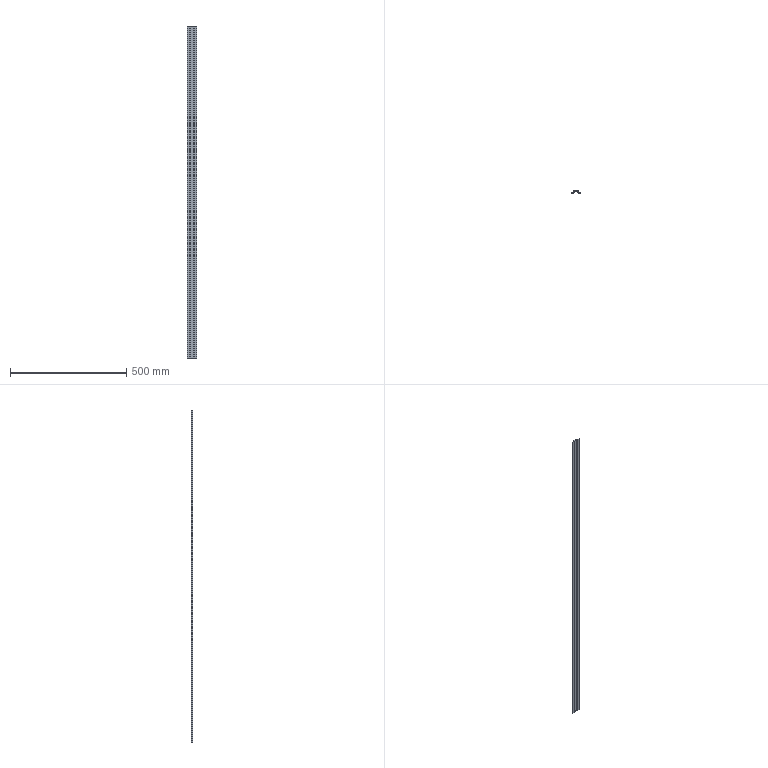Part | SolidWorks | features FlatPattern 1, SMBaseFlange 1, SheetMetal 1 | 1 solid | 38 faces | box 40 x 6.5 x 1430 mm | volume 103752 mm3 | plane 30 | cylinder 8 | commonest cylinder face diameters 0.4 x4 3.4 x4
STEP:
#1=CARTESIAN_POINT('',(10.,0.2,715.));
#2=VERTEX_POINT('',#1);
#3=CARTESIAN_POINT('',(11.5,0.2,715.));
#4=VERTEX_POINT('',#3);
#5=CARTESIAN_POINT('',(10.,0.2,715.));
#6=DIRECTION('',(1.,0.,0.));
#7=VECTOR('',#6,1000.);
#8=LINE('',#5,#7);
#9=EDGE_CURVE('',#2,#4,#8,.T.);
#10=ORIENTED_EDGE('',*,*,#9,.F.);
#11=CARTESIAN_POINT('',(9.8,0.,715.));
#12=VERTEX_POINT('',#11);
#13=CARTESIAN_POINT('',(9.8,0.2,715.));
#14=DIRECTION('',(0.,0.,1.));
#15=DIRECTION('',(-1.,0.,0.));
#16=AXIS2_PLACEMENT_3D('',#13,#14,#15);
#17=CIRCLE('',#16,0.2);
#18=EDGE_CURVE('',#12,#2,#17,.T.);
#19=ORIENTED_EDGE('',*,*,#18,.F.);
#20=CARTESIAN_POINT('',(9.8,-1.5,715.));
#21=VERTEX_POINT('',#20);
#22=CARTESIAN_POINT('',(9.8,-1.5,715.));
#23=DIRECTION('',(0.,1.,0.));
#24=VECTOR('',#23,1000.);
#25=LINE('',#22,#24);
#26=EDGE_CURVE('',#21,#12,#25,.T.);
#27=ORIENTED_EDGE('',*,*,#26,.F.);
#28=CARTESIAN_POINT('',(9.8,0.2,715.));
#29=DIRECTION('',(0.,0.,1.));
#30=DIRECTION('',(1.,0.,0.));
#31=AXIS2_PLACEMENT_3D('',#28,#29,#30);
#32=CIRCLE('',#31,1.7);
#33=EDGE_CURVE('',#21,#4,#32,.T.);
#34=ORIENTED_EDGE('',*,*,#33,.T.);
#35=EDGE_LOOP('',(#10,#19,#27,#34));
#36=FACE_OUTER_BOUND('',#35,.T.);
#37=CARTESIAN_POINT('',(10.,0.2,715.));
#38=DIRECTION('',(0.,0.,1.));
#39=DIRECTION('',(1.,0.,0.));
#40=AXIS2_PLACEMENT_3D('',#37,#38,#39);
#41=PLANE('',#40);
#42=ADVANCED_FACE('',(#36),#41,.T.);
#43=CARTESIAN_POINT('',(10.,3.3,715.));
#44=VERTEX_POINT('',#43);
#45=CARTESIAN_POINT('',(10.,0.,715.));
#46=DIRECTION('',(0.,1.,0.));
#47=VECTOR('',#46,1000.);
#48=LINE('',#45,#47);
#49=EDGE_CURVE('',#2,#44,#48,.T.);
#50=ORIENTED_EDGE('',*,*,#49,.F.);
#51=ORIENTED_EDGE('',*,*,#9,.T.);
#52=CARTESIAN_POINT('',(11.5,3.3,715.));
#53=VERTEX_POINT('',#52);
#54=CARTESIAN_POINT('',(11.5,0.,715.));
#55=DIRECTION('',(0.,1.,0.));
#56=VECTOR('',#55,1000.);
#57=LINE('',#54,#56);
#58=EDGE_CURVE('',#4,#53,#57,.T.);
#59=ORIENTED_EDGE('',*,*,#58,.T.);
#60=CARTESIAN_POINT('',(11.5,3.3,715.));
#61=DIRECTION('',(-1.,0.,0.));
#62=VECTOR('',#61,1000.);
#63=LINE('',#60,#62);
#64=EDGE_CURVE('',#53,#44,#63,.T.);
#65=ORIENTED_EDGE('',*,*,#64,.T.);
#66=EDGE_LOOP('',(#50,#51,#59,#65));
#67=FACE_OUTER_BOUND('',#66,.T.);
#68=CARTESIAN_POINT('',(9.8,-1.5,715.));
#69=DIRECTION('',(0.,0.,1.));
#70=DIRECTION('',(1.,0.,0.));
#71=AXIS2_PLACEMENT_3D('',#68,#69,#70);
#72=PLANE('',#71);
#73=ADVANCED_FACE('',(#67),#72,.T.);
#74=CARTESIAN_POINT('',(9.8,0.,-715.));
#75=VERTEX_POINT('',#74);
#76=CARTESIAN_POINT('',(9.8,-1.5,-715.));
#77=VERTEX_POINT('',#76);
#78=CARTESIAN_POINT('',(9.8,0.,-715.));
#79=DIRECTION('',(0.,-1.,0.));
#80=VECTOR('',#79,1000.);
#81=LINE('',#78,#80);
#82=EDGE_CURVE('',#75,#77,#81,.T.);
#83=ORIENTED_EDGE('',*,*,#82,.F.);
#84=CARTESIAN_POINT('',(10.,0.2,-715.));
#85=VERTEX_POINT('',#84);
#86=CARTESIAN_POINT('',(9.8,0.2,-715.));
#87=DIRECTION('',(0.,0.,1.));
#88=DIRECTION('',(-1.,0.,0.));
#89=AXIS2_PLACEMENT_3D('',#86,#87,#88);
#90=CIRCLE('',#89,0.2);
#91=EDGE_CURVE('',#75,#85,#90,.T.);
#92=ORIENTED_EDGE('',*,*,#91,.T.);
#93=CARTESIAN_POINT('',(11.5,0.2,-715.));
#94=VERTEX_POINT('',#93);
#95=CARTESIAN_POINT('',(11.5,0.2,-715.));
#96=DIRECTION('',(-1.,0.,0.));
#97=VECTOR('',#96,1000.);
#98=LINE('',#95,#97);
#99=EDGE_CURVE('',#94,#85,#98,.T.);
#100=ORIENTED_EDGE('',*,*,#99,.F.);
#101=CARTESIAN_POINT('',(9.8,0.2,-715.));
#102=DIRECTION('',(0.,0.,1.));
#103=DIRECTION('',(1.,0.,0.));
#104=AXIS2_PLACEMENT_3D('',#101,#102,#103);
#105=CIRCLE('',#104,1.7);
#106=EDGE_CURVE('',#77,#94,#105,.T.);
#107=ORIENTED_EDGE('',*,*,#106,.F.);
#108=EDGE_LOOP('',(#83,#92,#100,#107));
#109=FACE_OUTER_BOUND('',#108,.T.);
#110=CARTESIAN_POINT('',(9.8,0.,-715.));
#111=DIRECTION('',(0.,0.,-1.));
#112=DIRECTION('',(-1.,0.,0.));
#113=AXIS2_PLACEMENT_3D('',#110,#111,#112);
#114=PLANE('',#113);
#115=ADVANCED_FACE('',(#109),#114,.T.);
#116=CARTESIAN_POINT('',(0.,0.,-715.));
#117=VERTEX_POINT('',#116);
#118=CARTESIAN_POINT('',(0.,0.,-715.));
#119=DIRECTION('',(1.,0.,0.));
#120=VECTOR('',#119,1000.);
#121=LINE('',#118,#120);
#122=EDGE_CURVE('',#117,#75,#121,.T.);
#123=ORIENTED_EDGE('',*,*,#122,.T.);
#124=ORIENTED_EDGE('',*,*,#82,.T.);
#125=CARTESIAN_POINT('',(0.,-1.5,-715.));
#126=VERTEX_POINT('',#125);
#127=CARTESIAN_POINT('',(0.,-1.5,-715.));
#128=DIRECTION('',(1.,0.,0.));
#129=VECTOR('',#128,1000.);
#130=LINE('',#127,#129);
#131=EDGE_CURVE('',#126,#77,#130,.T.);
#132=ORIENTED_EDGE('',*,*,#131,.F.);
#133=CARTESIAN_POINT('',(0.,-1.5,-715.));
#134=DIRECTION('',(0.,1.,0.));
#135=VECTOR('',#134,1000.);
#136=LINE('',#133,#135);
#137=EDGE_CURVE('',#126,#117,#136,.T.);
#138=ORIENTED_EDGE('',*,*,#137,.T.);
#139=EDGE_LOOP('',(#123,#124,#132,#138));
#140=FACE_OUTER_BOUND('',#139,.T.);
#141=CARTESIAN_POINT('',(11.5,0.2,-715.));
#142=DIRECTION('',(0.,0.,-1.));
#143=DIRECTION('',(-1.,0.,0.));
#144=AXIS2_PLACEMENT_3D('',#141,#142,#143);
#145=PLANE('',#144);
#146=ADVANCED_FACE('',(#140),#145,.T.);
#147=CARTESIAN_POINT('',(11.7,5.,715.));
#148=VERTEX_POINT('',#147);
#149=CARTESIAN_POINT('',(11.7,3.5,715.));
#150=VERTEX_POINT('',#149);
#151=CARTESIAN_POINT('',(11.7,5.,715.));
#152=DIRECTION('',(0.,-1.,0.));
#153=VECTOR('',#152,1000.);
#154=LINE('',#151,#153);
#155=EDGE_CURVE('',#148,#150,#154,.T.);
#156=ORIENTED_EDGE('',*,*,#155,.F.);
#157=CARTESIAN_POINT('',(11.7,3.3,715.));
#158=DIRECTION('',(0.,0.,-1.));
#159=DIRECTION('',(1.,0.,0.));
#160=AXIS2_PLACEMENT_3D('',#157,#158,#159);
#161=CIRCLE('',#160,1.7);
#162=EDGE_CURVE('',#44,#148,#161,.T.);
#163=ORIENTED_EDGE('',*,*,#162,.F.);
#164=ORIENTED_EDGE('',*,*,#64,.F.);
#165=CARTESIAN_POINT('',(11.7,3.3,715.));
#166=DIRECTION('',(0.,0.,-1.));
#167=DIRECTION('',(1.,0.,0.));
#168=AXIS2_PLACEMENT_3D('',#165,#166,#167);
#169=CIRCLE('',#168,0.2);
#170=EDGE_CURVE('',#53,#150,#169,.T.);
#171=ORIENTED_EDGE('',*,*,#170,.T.);
#172=EDGE_LOOP('',(#156,#163,#164,#171));
#173=FACE_OUTER_BOUND('',#172,.T.);
#174=CARTESIAN_POINT('',(11.7,5.,715.));
#175=DIRECTION('',(0.,0.,1.));
#176=DIRECTION('',(1.,0.,0.));
#177=AXIS2_PLACEMENT_3D('',#174,#175,#176);
#178=PLANE('',#177);
#179=ADVANCED_FACE('',(#173),#178,.T.);
#180=CARTESIAN_POINT('',(28.3,5.,715.));
#181=VERTEX_POINT('',#180);
#182=CARTESIAN_POINT('',(10.,5.,715.));
#183=DIRECTION('',(1.,0.,0.));
#184=VECTOR('',#183,1000.);
#185=LINE('',#182,#184);
#186=EDGE_CURVE('',#148,#181,#185,.T.);
#187=ORIENTED_EDGE('',*,*,#186,.F.);
#188=ORIENTED_EDGE('',*,*,#155,.T.);
#189=CARTESIAN_POINT('',(28.3,3.5,715.));
#190=VERTEX_POINT('',#189);
#191=CARTESIAN_POINT('',(10.,3.5,715.));
#192=DIRECTION('',(1.,0.,0.));
#193=VECTOR('',#192,1000.);
#194=LINE('',#191,#193);
#195=EDGE_CURVE('',#150,#190,#194,.T.);
#196=ORIENTED_EDGE('',*,*,#195,.T.);
#197=CARTESIAN_POINT('',(28.3,3.5,715.));
#198=DIRECTION('',(0.,1.,0.));
#199=VECTOR('',#198,1000.);
#200=LINE('',#197,#199);
#201=EDGE_CURVE('',#190,#181,#200,.T.);
#202=ORIENTED_EDGE('',*,*,#201,.T.);
#203=EDGE_LOOP('',(#187,#188,#196,#202));
#204=FACE_OUTER_BOUND('',#203,.T.);
#205=CARTESIAN_POINT('',(11.5,3.3,715.));
#206=DIRECTION('',(0.,0.,1.));
#207=DIRECTION('',(1.,0.,0.));
#208=AXIS2_PLACEMENT_3D('',#205,#206,#207);
#209=PLANE('',#208);
#210=ADVANCED_FACE('',(#204),#209,.T.);
#211=CARTESIAN_POINT('',(10.,3.3,-715.));
#212=VERTEX_POINT('',#211);
#213=CARTESIAN_POINT('',(11.5,3.3,-715.));
#214=VERTEX_POINT('',#213);
#215=CARTESIAN_POINT('',(10.,3.3,-715.));
#216=DIRECTION('',(1.,0.,0.));
#217=VECTOR('',#216,1000.);
#218=LINE('',#215,#217);
#219=EDGE_CURVE('',#212,#214,#218,.T.);
#220=ORIENTED_EDGE('',*,*,#219,.F.);
#221=CARTESIAN_POINT('',(11.7,5.,-715.));
#222=VERTEX_POINT('',#221);
#223=CARTESIAN_POINT('',(11.7,3.3,-715.));
#224=DIRECTION('',(0.,0.,-1.));
#225=DIRECTION('',(1.,0.,0.));
#226=AXIS2_PLACEMENT_3D('',#223,#224,#225);
#227=CIRCLE('',#226,1.7);
#228=EDGE_CURVE('',#212,#222,#227,.T.);
#229=ORIENTED_EDGE('',*,*,#228,.T.);
#230=CARTESIAN_POINT('',(11.7,3.5,-715.));
#231=VERTEX_POINT('',#230);
#232=CARTESIAN_POINT('',(11.7,3.5,-715.));
#233=DIRECTION('',(0.,1.,0.));
#234=VECTOR('',#233,1000.);
#235=LINE('',#232,#234);
#236=EDGE_CURVE('',#231,#222,#235,.T.);
#237=ORIENTED_EDGE('',*,*,#236,.F.);
#238=CARTESIAN_POINT('',(11.7,3.3,-715.));
#239=DIRECTION('',(0.,0.,-1.));
#240=DIRECTION('',(1.,0.,0.));
#241=AXIS2_PLACEMENT_3D('',#238,#239,#240);
#242=CIRCLE('',#241,0.2);
#243=EDGE_CURVE('',#214,#231,#242,.T.);
#244=ORIENTED_EDGE('',*,*,#243,.F.);
#245=EDGE_LOOP('',(#220,#229,#237,#244));
#246=FACE_OUTER_BOUND('',#245,.T.);
#247=CARTESIAN_POINT('',(10.,3.3,-715.));
#248=DIRECTION('',(0.,0.,-1.));
#249=DIRECTION('',(-1.,0.,0.));
#250=AXIS2_PLACEMENT_3D('',#247,#248,#249);
#251=PLANE('',#250);
#252=ADVANCED_FACE('',(#246),#251,.T.);
#253=CARTESIAN_POINT('',(10.,0.,-715.));
#254=DIRECTION('',(0.,1.,0.));
#255=VECTOR('',#254,1000.);
#256=LINE('',#253,#255);
#257=EDGE_CURVE('',#85,#212,#256,.T.);
#258=ORIENTED_EDGE('',*,*,#257,.T.);
#259=ORIENTED_EDGE('',*,*,#219,.T.);
#260=CARTESIAN_POINT('',(11.5,0.,-715.));
#261=DIRECTION('',(0.,1.,0.));
#262=VECTOR('',#261,1000.);
#263=LINE('',#260,#262);
#264=EDGE_CURVE('',#94,#214,#263,.T.);
#265=ORIENTED_EDGE('',*,*,#264,.F.);
#266=ORIENTED_EDGE('',*,*,#99,.T.);
#267=EDGE_LOOP('',(#258,#259,#265,#266));
#268=FACE_OUTER_BOUND('',#267,.T.);
#269=CARTESIAN_POINT('',(11.7,3.5,-715.));
#270=DIRECTION('',(0.,0.,-1.));
#271=DIRECTION('',(-1.,0.,0.));
#272=AXIS2_PLACEMENT_3D('',#269,#270,#271);
#273=PLANE('',#272);
#274=ADVANCED_FACE('',(#268),#273,.T.);
#275=CARTESIAN_POINT('',(30.,3.3,715.));
#276=VERTEX_POINT('',#275);
#277=CARTESIAN_POINT('',(28.5,3.3,715.));
#278=VERTEX_POINT('',#277);
#279=CARTESIAN_POINT('',(30.,3.3,715.));
#280=DIRECTION('',(-1.,0.,0.));
#281=VECTOR('',#280,1000.);
#282=LINE('',#279,#281);
#283=EDGE_CURVE('',#276,#278,#282,.T.);
#284=ORIENTED_EDGE('',*,*,#283,.F.);
#285=CARTESIAN_POINT('',(28.3,3.3,715.));
#286=DIRECTION('',(0.,0.,-1.));
#287=DIRECTION('',(1.,0.,0.));
#288=AXIS2_PLACEMENT_3D('',#285,#286,#287);
#289=CIRCLE('',#288,1.7);
#290=EDGE_CURVE('',#181,#276,#289,.T.);
#291=ORIENTED_EDGE('',*,*,#290,.F.);
#292=ORIENTED_EDGE('',*,*,#201,.F.);
#293=CARTESIAN_POINT('',(28.3,3.3,715.));
#294=DIRECTION('',(0.,0.,-1.));
#295=DIRECTION('',(1.,0.,0.));
#296=AXIS2_PLACEMENT_3D('',#293,#294,#295);
#297=CIRCLE('',#296,0.2);
#298=EDGE_CURVE('',#190,#278,#297,.T.);
#299=ORIENTED_EDGE('',*,*,#298,.T.);
#300=EDGE_LOOP('',(#284,#291,#292,#299));
#301=FACE_OUTER_BOUND('',#300,.T.);
#302=CARTESIAN_POINT('',(30.,3.3,715.));
#303=DIRECTION('',(0.,0.,1.));
#304=DIRECTION('',(1.,0.,0.));
#305=AXIS2_PLACEMENT_3D('',#302,#303,#304);
#306=PLANE('',#305);
#307=ADVANCED_FACE('',(#301),#306,.T.);
#308=CARTESIAN_POINT('',(30.,0.2,715.));
#309=VERTEX_POINT('',#308);
#310=CARTESIAN_POINT('',(30.,5.,715.));
#311=DIRECTION('',(0.,-1.,0.));
#312=VECTOR('',#311,1000.);
#313=LINE('',#310,#312);
#314=EDGE_CURVE('',#276,#309,#313,.T.);
#315=ORIENTED_EDGE('',*,*,#314,.F.);
#316=ORIENTED_EDGE('',*,*,#283,.T.);
#317=CARTESIAN_POINT('',(28.5,0.2,715.));
#318=VERTEX_POINT('',#317);
#319=CARTESIAN_POINT('',(28.5,5.,715.));
#320=DIRECTION('',(0.,-1.,0.));
#321=VECTOR('',#320,1000.);
#322=LINE('',#319,#321);
#323=EDGE_CURVE('',#278,#318,#322,.T.);
#324=ORIENTED_EDGE('',*,*,#323,.T.);
#325=CARTESIAN_POINT('',(28.5,0.2,715.));
#326=DIRECTION('',(1.,0.,0.));
#327=VECTOR('',#326,1000.);
#328=LINE('',#325,#327);
#329=EDGE_CURVE('',#318,#309,#328,.T.);
#330=ORIENTED_EDGE('',*,*,#329,.T.);
#331=EDGE_LOOP('',(#315,#316,#324,#330));
#332=FACE_OUTER_BOUND('',#331,.T.);
#333=CARTESIAN_POINT('',(28.3,3.5,715.));
#334=DIRECTION('',(0.,0.,1.));
#335=DIRECTION('',(1.,0.,0.));
#336=AXIS2_PLACEMENT_3D('',#333,#334,#335);
#337=PLANE('',#336);
#338=ADVANCED_FACE('',(#332),#337,.T.);
#339=CARTESIAN_POINT('',(28.3,5.,-715.));
#340=VERTEX_POINT('',#339);
#341=CARTESIAN_POINT('',(28.3,3.5,-715.));
#342=VERTEX_POINT('',#341);
#343=CARTESIAN_POINT('',(28.3,5.,-715.));
#344=DIRECTION('',(0.,-1.,0.));
#345=VECTOR('',#344,1000.);
#346=LINE('',#343,#345);
#347=EDGE_CURVE('',#340,#342,#346,.T.);
#348=ORIENTED_EDGE('',*,*,#347,.F.);
#349=CARTESIAN_POINT('',(30.,3.3,-715.));
#350=VERTEX_POINT('',#349);
#351=CARTESIAN_POINT('',(28.3,3.3,-715.));
#352=DIRECTION('',(0.,0.,-1.));
#353=DIRECTION('',(1.,0.,0.));
#354=AXIS2_PLACEMENT_3D('',#351,#352,#353);
#355=CIRCLE('',#354,1.7);
#356=EDGE_CURVE('',#340,#350,#355,.T.);
#357=ORIENTED_EDGE('',*,*,#356,.T.);
#358=CARTESIAN_POINT('',(28.5,3.3,-715.));
#359=VERTEX_POINT('',#358);
#360=CARTESIAN_POINT('',(28.5,3.3,-715.));
#361=DIRECTION('',(1.,0.,0.));
#362=VECTOR('',#361,1000.);
#363=LINE('',#360,#362);
#364=EDGE_CURVE('',#359,#350,#363,.T.);
#365=ORIENTED_EDGE('',*,*,#364,.F.);
#366=CARTESIAN_POINT('',(28.3,3.3,-715.));
#367=DIRECTION('',(0.,0.,-1.));
#368=DIRECTION('',(1.,0.,0.));
#369=AXIS2_PLACEMENT_3D('',#366,#367,#368);
#370=CIRCLE('',#369,0.2);
#371=EDGE_CURVE('',#342,#359,#370,.T.);
#372=ORIENTED_EDGE('',*,*,#371,.F.);
#373=EDGE_LOOP('',(#348,#357,#365,#372));
#374=FACE_OUTER_BOUND('',#373,.T.);
#375=CARTESIAN_POINT('',(28.3,5.,-715.));
#376=DIRECTION('',(0.,0.,-1.));
#377=DIRECTION('',(-1.,0.,0.));
#378=AXIS2_PLACEMENT_3D('',#375,#376,#377);
#379=PLANE('',#378);
#380=ADVANCED_FACE('',(#374),#379,.T.);
#381=CARTESIAN_POINT('',(10.,5.,-715.));
#382=DIRECTION('',(1.,0.,0.));
#383=VECTOR('',#382,1000.);
#384=LINE('',#381,#383);
#385=EDGE_CURVE('',#222,#340,#384,.T.);
#386=ORIENTED_EDGE('',*,*,#385,.T.);
#387=ORIENTED_EDGE('',*,*,#347,.T.);
#388=CARTESIAN_POINT('',(10.,3.5,-715.));
#389=DIRECTION('',(1.,0.,0.));
#390=VECTOR('',#389,1000.);
#391=LINE('',#388,#390);
#392=EDGE_CURVE('',#231,#342,#391,.T.);
#393=ORIENTED_EDGE('',*,*,#392,.F.);
#394=ORIENTED_EDGE('',*,*,#236,.T.);
#395=EDGE_LOOP('',(#386,#387,#393,#394));
#396=FACE_OUTER_BOUND('',#395,.T.);
#397=CARTESIAN_POINT('',(28.5,3.3,-715.));
#398=DIRECTION('',(0.,0.,-1.));
#399=DIRECTION('',(-1.,0.,0.));
#400=AXIS2_PLACEMENT_3D('',#397,#398,#399);
#401=PLANE('',#400);
#402=ADVANCED_FACE('',(#396),#401,.T.);
#403=CARTESIAN_POINT('',(30.2,0.,715.));
#404=VERTEX_POINT('',#403);
#405=CARTESIAN_POINT('',(30.2,-1.5,715.));
#406=VERTEX_POINT('',#405);
#407=CARTESIAN_POINT('',(30.2,0.,715.));
#408=DIRECTION('',(0.,-1.,0.));
#409=VECTOR('',#408,1000.);
#410=LINE('',#407,#409);
#411=EDGE_CURVE('',#404,#406,#410,.T.);
#412=ORIENTED_EDGE('',*,*,#411,.F.);
#413=CARTESIAN_POINT('',(30.2,0.2,715.));
#414=DIRECTION('',(0.,0.,1.));
#415=DIRECTION('',(-1.,0.,0.));
#416=AXIS2_PLACEMENT_3D('',#413,#414,#415);
#417=CIRCLE('',#416,0.2);
#418=EDGE_CURVE('',#309,#404,#417,.T.);
#419=ORIENTED_EDGE('',*,*,#418,.F.);
#420=ORIENTED_EDGE('',*,*,#329,.F.);
#421=CARTESIAN_POINT('',(30.2,0.2,715.));
#422=DIRECTION('',(0.,0.,1.));
#423=DIRECTION('',(1.,0.,0.));
#424=AXIS2_PLACEMENT_3D('',#421,#422,#423);
#425=CIRCLE('',#424,1.7);
#426=EDGE_CURVE('',#318,#406,#425,.T.);
#427=ORIENTED_EDGE('',*,*,#426,.T.);
#428=EDGE_LOOP('',(#412,#419,#420,#427));
#429=FACE_OUTER_BOUND('',#428,.T.);
#430=CARTESIAN_POINT('',(30.2,0.,715.));
#431=DIRECTION('',(0.,0.,1.));
#432=DIRECTION('',(1.,0.,0.));
#433=AXIS2_PLACEMENT_3D('',#430,#431,#432);
#434=PLANE('',#433);
#435=ADVANCED_FACE('',(#429),#434,.T.);
#436=CARTESIAN_POINT('',(40.,0.,715.));
#437=VERTEX_POINT('',#436);
#438=CARTESIAN_POINT('',(30.,0.,715.));
#439=DIRECTION('',(1.,0.,0.));
#440=VECTOR('',#439,1000.);
#441=LINE('',#438,#440);
#442=EDGE_CURVE('',#404,#437,#441,.T.);
#443=ORIENTED_EDGE('',*,*,#442,.F.);
#444=ORIENTED_EDGE('',*,*,#411,.T.);
#445=CARTESIAN_POINT('',(40.,-1.5,715.));
#446=VERTEX_POINT('',#445);
#447=CARTESIAN_POINT('',(30.,-1.5,715.));
#448=DIRECTION('',(1.,0.,0.));
#449=VECTOR('',#448,1000.);
#450=LINE('',#447,#449);
#451=EDGE_CURVE('',#406,#446,#450,.T.);
#452=ORIENTED_EDGE('',*,*,#451,.T.);
#453=CARTESIAN_POINT('',(40.,0.,715.));
#454=DIRECTION('',(0.,-1.,0.));
#455=VECTOR('',#454,1000.);
#456=LINE('',#453,#455);
#457=EDGE_CURVE('',#437,#446,#456,.T.);
#458=ORIENTED_EDGE('',*,*,#457,.F.);
#459=EDGE_LOOP('',(#443,#444,#452,#458));
#460=FACE_OUTER_BOUND('',#459,.T.);
#461=CARTESIAN_POINT('',(28.5,0.2,715.));
#462=DIRECTION('',(0.,0.,1.));
#463=DIRECTION('',(1.,0.,0.));
#464=AXIS2_PLACEMENT_3D('',#461,#462,#463);
#465=PLANE('',#464);
#466=ADVANCED_FACE('',(#460),#465,.T.);
#467=CARTESIAN_POINT('',(30.,0.2,-715.));
#468=VERTEX_POINT('',#467);
#469=CARTESIAN_POINT('',(28.5,0.2,-715.));
#470=VERTEX_POINT('',#469);
#471=CARTESIAN_POINT('',(30.,0.2,-715.));
#472=DIRECTION('',(-1.,0.,0.));
#473=VECTOR('',#472,1000.);
#474=LINE('',#471,#473);
#475=EDGE_CURVE('',#468,#470,#474,.T.);
#476=ORIENTED_EDGE('',*,*,#475,.F.);
#477=CARTESIAN_POINT('',(30.2,0.,-715.));
#478=VERTEX_POINT('',#477);
#479=CARTESIAN_POINT('',(30.2,0.2,-715.));
#480=DIRECTION('',(0.,0.,1.));
#481=DIRECTION('',(-1.,0.,0.));
#482=AXIS2_PLACEMENT_3D('',#479,#480,#481);
#483=CIRCLE('',#482,0.2);
#484=EDGE_CURVE('',#468,#478,#483,.T.);
#485=ORIENTED_EDGE('',*,*,#484,.T.);
#486=CARTESIAN_POINT('',(30.2,-1.5,-715.));
#487=VERTEX_POINT('',#486);
#488=CARTESIAN_POINT('',(30.2,-1.5,-715.));
#489=DIRECTION('',(0.,1.,0.));
#490=VECTOR('',#489,1000.);
#491=LINE('',#488,#490);
#492=EDGE_CURVE('',#487,#478,#491,.T.);
#493=ORIENTED_EDGE('',*,*,#492,.F.);
#494=CARTESIAN_POINT('',(30.2,0.2,-715.));
#495=DIRECTION('',(0.,0.,1.));
#496=DIRECTION('',(1.,0.,0.));
#497=AXIS2_PLACEMENT_3D('',#494,#495,#496);
#498=CIRCLE('',#497,1.7);
#499=EDGE_CURVE('',#470,#487,#498,.T.);
#500=ORIENTED_EDGE('',*,*,#499,.F.);
#501=EDGE_LOOP('',(#476,#485,#493,#500));
#502=FACE_OUTER_BOUND('',#501,.T.);
#503=CARTESIAN_POINT('',(30.,0.2,-715.));
#504=DIRECTION('',(0.,0.,-1.));
#505=DIRECTION('',(-1.,0.,0.));
#506=AXIS2_PLACEMENT_3D('',#503,#504,#505);
#507=PLANE('',#506);
#508=ADVANCED_FACE('',(#502),#507,.T.);
#509=CARTESIAN_POINT('',(30.,5.,-715.));
#510=DIRECTION('',(0.,-1.,0.));
#511=VECTOR('',#510,1000.);
#512=LINE('',#509,#511);
#513=EDGE_CURVE('',#350,#468,#512,.T.);
#514=ORIENTED_EDGE('',*,*,#513,.T.);
#515=ORIENTED_EDGE('',*,*,#475,.T.);
#516=CARTESIAN_POINT('',(28.5,5.,-715.));
#517=DIRECTION('',(0.,-1.,0.));
#518=VECTOR('',#517,1000.);
#519=LINE('',#516,#518);
#520=EDGE_CURVE('',#359,#470,#519,.T.);
#521=ORIENTED_EDGE('',*,*,#520,.F.);
#522=ORIENTED_EDGE('',*,*,#364,.T.);
#523=EDGE_LOOP('',(#514,#515,#521,#522));
#524=FACE_OUTER_BOUND('',#523,.T.);
#525=CARTESIAN_POINT('',(30.2,-1.5,-715.));
#526=DIRECTION('',(0.,0.,-1.));
#527=DIRECTION('',(-1.,0.,0.));
#528=AXIS2_PLACEMENT_3D('',#525,#526,#527);
#529=PLANE('',#528);
#530=ADVANCED_FACE('',(#524),#529,.T.);
#531=CARTESIAN_POINT('',(40.,-1.5,-715.));
#532=VERTEX_POINT('',#531);
#533=CARTESIAN_POINT('',(30.,-1.5,-715.));
#534=DIRECTION('',(1.,0.,0.));
#535=VECTOR('',#534,1000.);
#536=LINE('',#533,#535);
#537=EDGE_CURVE('',#487,#532,#536,.T.);
#538=ORIENTED_EDGE('',*,*,#537,.T.);
#539=CARTESIAN_POINT('',(40.,-1.5,715.));
#540=DIRECTION('',(0.,0.,-1.));
#541=VECTOR('',#540,1000.);
#542=LINE('',#539,#541);
#543=EDGE_CURVE('',#446,#532,#542,.T.);
#544=ORIENTED_EDGE('',*,*,#543,.F.);
#545=ORIENTED_EDGE('',*,*,#451,.F.);
#546=CARTESIAN_POINT('',(30.2,-1.5,715.));
#547=DIRECTION('',(0.,0.,-1.));
#548=VECTOR('',#547,1000.);
#549=LINE('',#546,#548);
#550=EDGE_CURVE('',#406,#487,#549,.T.);
#551=ORIENTED_EDGE('',*,*,#550,.T.);
#552=EDGE_LOOP('',(#538,#544,#545,#551));
#553=FACE_OUTER_BOUND('',#552,.T.);
#554=CARTESIAN_POINT('',(30.,-1.5,715.));
#555=DIRECTION('',(0.,1.,0.));
#556=DIRECTION('',(0.,0.,1.));
#557=AXIS2_PLACEMENT_3D('',#554,#555,#556);
#558=PLANE('',#557);
#559=ADVANCED_FACE('',(#553),#558,.F.);
#560=CARTESIAN_POINT('',(40.,0.,-715.));
#561=VERTEX_POINT('',#560);
#562=CARTESIAN_POINT('',(40.,0.,-715.));
#563=DIRECTION('',(0.,-1.,0.));
#564=VECTOR('',#563,1000.);
#565=LINE('',#562,#564);
#566=EDGE_CURVE('',#561,#532,#565,.T.);
#567=ORIENTED_EDGE('',*,*,#566,.F.);
#568=CARTESIAN_POINT('',(40.,0.,715.));
#569=DIRECTION('',(0.,0.,-1.));
#570=VECTOR('',#569,1000.);
#571=LINE('',#568,#570);
#572=EDGE_CURVE('',#437,#561,#571,.T.);
#573=ORIENTED_EDGE('',*,*,#572,.F.);
#574=ORIENTED_EDGE('',*,*,#457,.T.);
#575=ORIENTED_EDGE('',*,*,#543,.T.);
#576=EDGE_LOOP('',(#567,#573,#574,#575));
#577=FACE_OUTER_BOUND('',#576,.T.);
#578=CARTESIAN_POINT('',(40.,0.,715.));
#579=DIRECTION('',(1.,0.,0.));
#580=DIRECTION('',(0.,0.,-1.));
#581=AXIS2_PLACEMENT_3D('',#578,#579,#580);
#582=PLANE('',#581);
#583=ADVANCED_FACE('',(#577),#582,.T.);
#584=CARTESIAN_POINT('',(30.,0.,-715.));
#585=DIRECTION('',(1.,0.,0.));
#586=VECTOR('',#585,1000.);
#587=LINE('',#584,#586);
#588=EDGE_CURVE('',#478,#561,#587,.T.);
#589=ORIENTED_EDGE('',*,*,#588,.F.);
#590=CARTESIAN_POINT('',(30.2,0.,715.));
#591=DIRECTION('',(0.,0.,-1.));
#592=VECTOR('',#591,1000.);
#593=LINE('',#590,#592);
#594=EDGE_CURVE('',#404,#478,#593,.T.);
#595=ORIENTED_EDGE('',*,*,#594,.F.);
#596=ORIENTED_EDGE('',*,*,#442,.T.);
#597=ORIENTED_EDGE('',*,*,#572,.T.);
#598=EDGE_LOOP('',(#589,#595,#596,#597));
#599=FACE_OUTER_BOUND('',#598,.T.);
#600=CARTESIAN_POINT('',(30.,0.,715.));
#601=DIRECTION('',(0.,1.,0.));
#602=DIRECTION('',(0.,0.,1.));
#603=AXIS2_PLACEMENT_3D('',#600,#601,#602);
#604=PLANE('',#603);
#605=ADVANCED_FACE('',(#599),#604,.T.);
#606=ORIENTED_EDGE('',*,*,#484,.F.);
#607=CARTESIAN_POINT('',(30.,0.2,715.));
#608=DIRECTION('',(0.,0.,-1.));
#609=VECTOR('',#608,1000.);
#610=LINE('',#607,#609);
#611=EDGE_CURVE('',#309,#468,#610,.T.);
#612=ORIENTED_EDGE('',*,*,#611,.F.);
#613=ORIENTED_EDGE('',*,*,#418,.T.);
#614=ORIENTED_EDGE('',*,*,#594,.T.);
#615=EDGE_LOOP('',(#606,#612,#613,#614));
#616=FACE_OUTER_BOUND('',#615,.T.);
#617=CARTESIAN_POINT('',(30.2,0.2,715.));
#618=DIRECTION('',(0.,0.,-1.));
#619=DIRECTION('',(-1.,0.,0.));
#620=AXIS2_PLACEMENT_3D('',#617,#618,#619);
#621=CYLINDRICAL_SURFACE('',#620,0.2);
#622=ADVANCED_FACE('',(#616),#621,.F.);
#623=ORIENTED_EDGE('',*,*,#513,.F.);
#624=CARTESIAN_POINT('',(30.,3.3,715.));
#625=DIRECTION('',(0.,0.,-1.));
#626=VECTOR('',#625,1000.);
#627=LINE('',#624,#626);
#628=EDGE_CURVE('',#276,#350,#627,.T.);
#629=ORIENTED_EDGE('',*,*,#628,.F.);
#630=ORIENTED_EDGE('',*,*,#314,.T.);
#631=ORIENTED_EDGE('',*,*,#611,.T.);
#632=EDGE_LOOP('',(#623,#629,#630,#631));
#633=FACE_OUTER_BOUND('',#632,.T.);
#634=CARTESIAN_POINT('',(30.,5.,715.));
#635=DIRECTION('',(1.,0.,0.));
#636=DIRECTION('',(0.,0.,-1.));
#637=AXIS2_PLACEMENT_3D('',#634,#635,#636);
#638=PLANE('',#637);
#639=ADVANCED_FACE('',(#633),#638,.T.);
#640=ORIENTED_EDGE('',*,*,#356,.F.);
#641=CARTESIAN_POINT('',(28.3,5.,715.));
#642=DIRECTION('',(0.,0.,-1.));
#643=VECTOR('',#642,1000.);
#644=LINE('',#641,#643);
#645=EDGE_CURVE('',#181,#340,#644,.T.);
#646=ORIENTED_EDGE('',*,*,#645,.F.);
#647=ORIENTED_EDGE('',*,*,#290,.T.);
#648=ORIENTED_EDGE('',*,*,#628,.T.);
#649=EDGE_LOOP('',(#640,#646,#647,#648));
#650=FACE_OUTER_BOUND('',#649,.T.);
#651=CARTESIAN_POINT('',(28.3,3.3,715.));
#652=DIRECTION('',(0.,0.,-1.));
#653=DIRECTION('',(-1.,0.,0.));
#654=AXIS2_PLACEMENT_3D('',#651,#652,#653);
#655=CYLINDRICAL_SURFACE('',#654,1.7);
#656=ADVANCED_FACE('',(#650),#655,.T.);
#657=ORIENTED_EDGE('',*,*,#385,.F.);
#658=CARTESIAN_POINT('',(11.7,5.,715.));
#659=DIRECTION('',(0.,0.,-1.));
#660=VECTOR('',#659,1000.);
#661=LINE('',#658,#660);
#662=EDGE_CURVE('',#148,#222,#661,.T.);
#663=ORIENTED_EDGE('',*,*,#662,.F.);
#664=ORIENTED_EDGE('',*,*,#186,.T.);
#665=ORIENTED_EDGE('',*,*,#645,.T.);
#666=EDGE_LOOP('',(#657,#663,#664,#665));
#667=FACE_OUTER_BOUND('',#666,.T.);
#668=CARTESIAN_POINT('',(10.,5.,715.));
#669=DIRECTION('',(0.,1.,0.));
#670=DIRECTION('',(0.,0.,1.));
#671=AXIS2_PLACEMENT_3D('',#668,#669,#670);
#672=PLANE('',#671);
#673=ADVANCED_FACE('',(#667),#672,.T.);
#674=ORIENTED_EDGE('',*,*,#228,.F.);
#675=CARTESIAN_POINT('',(10.,3.3,715.));
#676=DIRECTION('',(0.,0.,-1.));
#677=VECTOR('',#676,1000.);
#678=LINE('',#675,#677);
#679=EDGE_CURVE('',#44,#212,#678,.T.);
#680=ORIENTED_EDGE('',*,*,#679,.F.);
#681=ORIENTED_EDGE('',*,*,#162,.T.);
#682=ORIENTED_EDGE('',*,*,#662,.T.);
#683=EDGE_LOOP('',(#674,#680,#681,#682));
#684=FACE_OUTER_BOUND('',#683,.T.);
#685=CARTESIAN_POINT('',(11.7,3.3,715.));
#686=DIRECTION('',(0.,0.,-1.));
#687=DIRECTION('',(-1.,0.,0.));
#688=AXIS2_PLACEMENT_3D('',#685,#686,#687);
#689=CYLINDRICAL_SURFACE('',#688,1.7);
#690=ADVANCED_FACE('',(#684),#689,.T.);
#691=ORIENTED_EDGE('',*,*,#257,.F.);
#692=CARTESIAN_POINT('',(10.,0.2,715.));
#693=DIRECTION('',(0.,0.,-1.));
#694=VECTOR('',#693,1000.);
#695=LINE('',#692,#694);
#696=EDGE_CURVE('',#2,#85,#695,.T.);
#697=ORIENTED_EDGE('',*,*,#696,.F.);
#698=ORIENTED_EDGE('',*,*,#49,.T.);
#699=ORIENTED_EDGE('',*,*,#679,.T.);
#700=EDGE_LOOP('',(#691,#697,#698,#699));
#701=FACE_OUTER_BOUND('',#700,.T.);
#702=CARTESIAN_POINT('',(10.,0.,715.));
#703=DIRECTION('',(-1.,0.,0.));
#704=DIRECTION('',(0.,0.,1.));
#705=AXIS2_PLACEMENT_3D('',#702,#703,#704);
#706=PLANE('',#705);
#707=ADVANCED_FACE('',(#701),#706,.T.);
#708=ORIENTED_EDGE('',*,*,#91,.F.);
#709=CARTESIAN_POINT('',(9.8,0.,715.));
#710=DIRECTION('',(0.,0.,-1.));
#711=VECTOR('',#710,1000.);
#712=LINE('',#709,#711);
#713=EDGE_CURVE('',#12,#75,#712,.T.);
#714=ORIENTED_EDGE('',*,*,#713,.F.);
#715=ORIENTED_EDGE('',*,*,#18,.T.);
#716=ORIENTED_EDGE('',*,*,#696,.T.);
#717=EDGE_LOOP('',(#708,#714,#715,#716));
#718=FACE_OUTER_BOUND('',#717,.T.);
#719=CARTESIAN_POINT('',(9.8,0.2,715.));
#720=DIRECTION('',(0.,0.,-1.));
#721=DIRECTION('',(-1.,0.,0.));
#722=AXIS2_PLACEMENT_3D('',#719,#720,#721);
#723=CYLINDRICAL_SURFACE('',#722,0.2);
#724=ADVANCED_FACE('',(#718),#723,.F.);
#725=ORIENTED_EDGE('',*,*,#122,.F.);
#726=CARTESIAN_POINT('',(0.,0.,715.));
#727=VERTEX_POINT('',#726);
#728=CARTESIAN_POINT('',(0.,0.,715.));
#729=DIRECTION('',(0.,0.,-1.));
#730=VECTOR('',#729,1000.);
#731=LINE('',#728,#730);
#732=EDGE_CURVE('',#727,#117,#731,.T.);
#733=ORIENTED_EDGE('',*,*,#732,.F.);
#734=CARTESIAN_POINT('',(0.,0.,715.));
#735=DIRECTION('',(1.,0.,0.));
#736=VECTOR('',#735,1000.);
#737=LINE('',#734,#736);
#738=EDGE_CURVE('',#727,#12,#737,.T.);
#739=ORIENTED_EDGE('',*,*,#738,.T.);
#740=ORIENTED_EDGE('',*,*,#713,.T.);
#741=EDGE_LOOP('',(#725,#733,#739,#740));
#742=FACE_OUTER_BOUND('',#741,.T.);
#743=CARTESIAN_POINT('',(0.,0.,715.));
#744=DIRECTION('',(0.,1.,0.));
#745=DIRECTION('',(0.,0.,1.));
#746=AXIS2_PLACEMENT_3D('',#743,#744,#745);
#747=PLANE('',#746);
#748=ADVANCED_FACE('',(#742),#747,.T.);
#749=ORIENTED_EDGE('',*,*,#137,.F.);
#750=CARTESIAN_POINT('',(0.,-1.5,715.));
#751=VERTEX_POINT('',#750);
#752=CARTESIAN_POINT('',(0.,-1.5,715.));
#753=DIRECTION('',(0.,0.,-1.));
#754=VECTOR('',#753,1000.);
#755=LINE('',#752,#754);
#756=EDGE_CURVE('',#751,#126,#755,.T.);
#757=ORIENTED_EDGE('',*,*,#756,.F.);
#758=CARTESIAN_POINT('',(0.,-1.5,715.));
#759=DIRECTION('',(0.,1.,0.));
#760=VECTOR('',#759,1000.);
#761=LINE('',#758,#760);
#762=EDGE_CURVE('',#751,#727,#761,.T.);
#763=ORIENTED_EDGE('',*,*,#762,.T.);
#764=ORIENTED_EDGE('',*,*,#732,.T.);
#765=EDGE_LOOP('',(#749,#757,#763,#764));
#766=FACE_OUTER_BOUND('',#765,.T.);
#767=CARTESIAN_POINT('',(0.,-1.5,715.));
#768=DIRECTION('',(-1.,0.,0.));
#769=DIRECTION('',(0.,0.,1.));
#770=AXIS2_PLACEMENT_3D('',#767,#768,#769);
#771=PLANE('',#770);
#772=ADVANCED_FACE('',(#766),#771,.T.);
#773=ORIENTED_EDGE('',*,*,#131,.T.);
#774=CARTESIAN_POINT('',(9.8,-1.5,715.));
#775=DIRECTION('',(0.,0.,-1.));
#776=VECTOR('',#775,1000.);
#777=LINE('',#774,#776);
#778=EDGE_CURVE('',#21,#77,#777,.T.);
#779=ORIENTED_EDGE('',*,*,#778,.F.);
#780=CARTESIAN_POINT('',(0.,-1.5,715.));
#781=DIRECTION('',(1.,0.,0.));
#782=VECTOR('',#781,1000.);
#783=LINE('',#780,#782);
#784=EDGE_CURVE('',#751,#21,#783,.T.);
#785=ORIENTED_EDGE('',*,*,#784,.F.);
#786=ORIENTED_EDGE('',*,*,#756,.T.);
#787=EDGE_LOOP('',(#773,#779,#785,#786));
#788=FACE_OUTER_BOUND('',#787,.T.);
#789=CARTESIAN_POINT('',(0.,-1.5,715.));
#790=DIRECTION('',(0.,1.,0.));
#791=DIRECTION('',(0.,0.,1.));
#792=AXIS2_PLACEMENT_3D('',#789,#790,#791);
#793=PLANE('',#792);
#794=ADVANCED_FACE('',(#788),#793,.F.);
#795=ORIENTED_EDGE('',*,*,#106,.T.);
#796=CARTESIAN_POINT('',(11.5,0.2,715.));
#797=DIRECTION('',(0.,0.,-1.));
#798=VECTOR('',#797,1000.);
#799=LINE('',#796,#798);
#800=EDGE_CURVE('',#4,#94,#799,.T.);
#801=ORIENTED_EDGE('',*,*,#800,.F.);
#802=ORIENTED_EDGE('',*,*,#33,.F.);
#803=ORIENTED_EDGE('',*,*,#778,.T.);
#804=EDGE_LOOP('',(#795,#801,#802,#803));
#805=FACE_OUTER_BOUND('',#804,.T.);
#806=CARTESIAN_POINT('',(9.8,0.2,715.));
#807=DIRECTION('',(0.,0.,-1.));
#808=DIRECTION('',(-1.,0.,0.));
#809=AXIS2_PLACEMENT_3D('',#806,#807,#808);
#810=CYLINDRICAL_SURFACE('',#809,1.7);
#811=ADVANCED_FACE('',(#805),#810,.T.);
#812=ORIENTED_EDGE('',*,*,#264,.T.);
#813=CARTESIAN_POINT('',(11.5,3.3,715.));
#814=DIRECTION('',(0.,0.,-1.));
#815=VECTOR('',#814,1000.);
#816=LINE('',#813,#815);
#817=EDGE_CURVE('',#53,#214,#816,.T.);
#818=ORIENTED_EDGE('',*,*,#817,.F.);
#819=ORIENTED_EDGE('',*,*,#58,.F.);
#820=ORIENTED_EDGE('',*,*,#800,.T.);
#821=EDGE_LOOP('',(#812,#818,#819,#820));
#822=FACE_OUTER_BOUND('',#821,.T.);
#823=CARTESIAN_POINT('',(11.5,0.,715.));
#824=DIRECTION('',(-1.,0.,0.));
#825=DIRECTION('',(0.,0.,1.));
#826=AXIS2_PLACEMENT_3D('',#823,#824,#825);
#827=PLANE('',#826);
#828=ADVANCED_FACE('',(#822),#827,.F.);
#829=ORIENTED_EDGE('',*,*,#243,.T.);
#830=CARTESIAN_POINT('',(11.7,3.5,715.));
#831=DIRECTION('',(0.,0.,-1.));
#832=VECTOR('',#831,1000.);
#833=LINE('',#830,#832);
#834=EDGE_CURVE('',#150,#231,#833,.T.);
#835=ORIENTED_EDGE('',*,*,#834,.F.);
#836=ORIENTED_EDGE('',*,*,#170,.F.);
#837=ORIENTED_EDGE('',*,*,#817,.T.);
#838=EDGE_LOOP('',(#829,#835,#836,#837));
#839=FACE_OUTER_BOUND('',#838,.T.);
#840=CARTESIAN_POINT('',(11.7,3.3,715.));
#841=DIRECTION('',(0.,0.,-1.));
#842=DIRECTION('',(-1.,0.,0.));
#843=AXIS2_PLACEMENT_3D('',#840,#841,#842);
#844=CYLINDRICAL_SURFACE('',#843,0.2);
#845=ADVANCED_FACE('',(#839),#844,.F.);
#846=ORIENTED_EDGE('',*,*,#392,.T.);
#847=CARTESIAN_POINT('',(28.3,3.5,715.));
#848=DIRECTION('',(0.,0.,-1.));
#849=VECTOR('',#848,1000.);
#850=LINE('',#847,#849);
#851=EDGE_CURVE('',#190,#342,#850,.T.);
#852=ORIENTED_EDGE('',*,*,#851,.F.);
#853=ORIENTED_EDGE('',*,*,#195,.F.);
#854=ORIENTED_EDGE('',*,*,#834,.T.);
#855=EDGE_LOOP('',(#846,#852,#853,#854));
#856=FACE_OUTER_BOUND('',#855,.T.);
#857=CARTESIAN_POINT('',(10.,3.5,715.));
#858=DIRECTION('',(0.,1.,0.));
#859=DIRECTION('',(0.,0.,1.));
#860=AXIS2_PLACEMENT_3D('',#857,#858,#859);
#861=PLANE('',#860);
#862=ADVANCED_FACE('',(#856),#861,.F.);
#863=ORIENTED_EDGE('',*,*,#371,.T.);
#864=CARTESIAN_POINT('',(28.5,3.3,715.));
#865=DIRECTION('',(0.,0.,-1.));
#866=VECTOR('',#865,1000.);
#867=LINE('',#864,#866);
#868=EDGE_CURVE('',#278,#359,#867,.T.);
#869=ORIENTED_EDGE('',*,*,#868,.F.);
#870=ORIENTED_EDGE('',*,*,#298,.F.);
#871=ORIENTED_EDGE('',*,*,#851,.T.);
#872=EDGE_LOOP('',(#863,#869,#870,#871));
#873=FACE_OUTER_BOUND('',#872,.T.);
#874=CARTESIAN_POINT('',(28.3,3.3,715.));
#875=DIRECTION('',(0.,0.,-1.));
#876=DIRECTION('',(-1.,0.,0.));
#877=AXIS2_PLACEMENT_3D('',#874,#875,#876);
#878=CYLINDRICAL_SURFACE('',#877,0.2);
#879=ADVANCED_FACE('',(#873),#878,.F.);
#880=ORIENTED_EDGE('',*,*,#520,.T.);
#881=CARTESIAN_POINT('',(28.5,0.2,715.));
#882=DIRECTION('',(0.,0.,-1.));
#883=VECTOR('',#882,1000.);
#884=LINE('',#881,#883);
#885=EDGE_CURVE('',#318,#470,#884,.T.);
#886=ORIENTED_EDGE('',*,*,#885,.F.);
#887=ORIENTED_EDGE('',*,*,#323,.F.);
#888=ORIENTED_EDGE('',*,*,#868,.T.);
#889=EDGE_LOOP('',(#880,#886,#887,#888));
#890=FACE_OUTER_BOUND('',#889,.T.);
#891=CARTESIAN_POINT('',(28.5,5.,715.));
#892=DIRECTION('',(1.,0.,0.));
#893=DIRECTION('',(0.,0.,-1.));
#894=AXIS2_PLACEMENT_3D('',#891,#892,#893);
#895=PLANE('',#894);
#896=ADVANCED_FACE('',(#890),#895,.F.);
#897=ORIENTED_EDGE('',*,*,#499,.T.);
#898=ORIENTED_EDGE('',*,*,#550,.F.);
#899=ORIENTED_EDGE('',*,*,#426,.F.);
#900=ORIENTED_EDGE('',*,*,#885,.T.);
#901=EDGE_LOOP('',(#897,#898,#899,#900));
#902=FACE_OUTER_BOUND('',#901,.T.);
#903=CARTESIAN_POINT('',(30.2,0.2,715.));
#904=DIRECTION('',(0.,0.,-1.));
#905=DIRECTION('',(-1.,0.,0.));
#906=AXIS2_PLACEMENT_3D('',#903,#904,#905);
#907=CYLINDRICAL_SURFACE('',#906,1.7);
#908=ADVANCED_FACE('',(#902),#907,.T.);
#909=ORIENTED_EDGE('',*,*,#784,.T.);
#910=ORIENTED_EDGE('',*,*,#26,.T.);
#911=ORIENTED_EDGE('',*,*,#738,.F.);
#912=ORIENTED_EDGE('',*,*,#762,.F.);
#913=EDGE_LOOP('',(#909,#910,#911,#912));
#914=FACE_OUTER_BOUND('',#913,.T.);
#915=CARTESIAN_POINT('',(30.2,0.2,715.));
#916=DIRECTION('',(0.,0.,-1.));
#917=DIRECTION('',(-1.,0.,0.));
#918=AXIS2_PLACEMENT_3D('',#915,#916,#917);
#919=PLANE('',#918);
#920=ADVANCED_FACE('',(#914),#919,.F.);
#921=ORIENTED_EDGE('',*,*,#537,.F.);
#922=ORIENTED_EDGE('',*,*,#492,.T.);
#923=ORIENTED_EDGE('',*,*,#588,.T.);
#924=ORIENTED_EDGE('',*,*,#566,.T.);
#925=EDGE_LOOP('',(#921,#922,#923,#924));
#926=FACE_OUTER_BOUND('',#925,.T.);
#927=CARTESIAN_POINT('',(30.2,0.2,-715.));
#928=DIRECTION('',(0.,0.,-1.));
#929=DIRECTION('',(-1.,0.,0.));
#930=AXIS2_PLACEMENT_3D('',#927,#928,#929);
#931=PLANE('',#930);
#932=ADVANCED_FACE('',(#926),#931,.T.);
#933=CLOSED_SHELL('',(#42,#73,#115,#146,#179,#210,#252,#274,#307,#338,#380,#402,#435,#466,#508,#530,#559,#583,#605,#622,#639,#656,#673,#690,#707,#724,#748,#772,#794,#811,#828,#845,#862,#879,#896,#908,#920,#932));
#934=MANIFOLD_SOLID_BREP('',#933);
#935=CARTESIAN_POINT('',(0.,0.,0.));
#936=DIRECTION('',(0.,0.,1.));
#937=DIRECTION('',(1.,0.,0.));
#938=AXIS2_PLACEMENT_3D('',#935,#936,#937);
#939=(LENGTH_UNIT()NAMED_UNIT(*)SI_UNIT(.MILLI.,.METRE.));
#940=UNCERTAINTY_MEASURE_WITH_UNIT(LENGTH_MEASURE(0.00001),#939,'','');
#941=(NAMED_UNIT(*)PLANE_ANGLE_UNIT()SI_UNIT($,.RADIAN.));
#942=(NAMED_UNIT(*)SI_UNIT($,.STERADIAN.)SOLID_ANGLE_UNIT());
#943=(GEOMETRIC_REPRESENTATION_CONTEXT(3)GLOBAL_UNCERTAINTY_ASSIGNED_CONTEXT((#940))GLOBAL_UNIT_ASSIGNED_CONTEXT((#939,#941,#942))REPRESENTATION_CONTEXT('',''));
#944=ADVANCED_BREP_SHAPE_REPRESENTATION('',(#934,#938),#943);